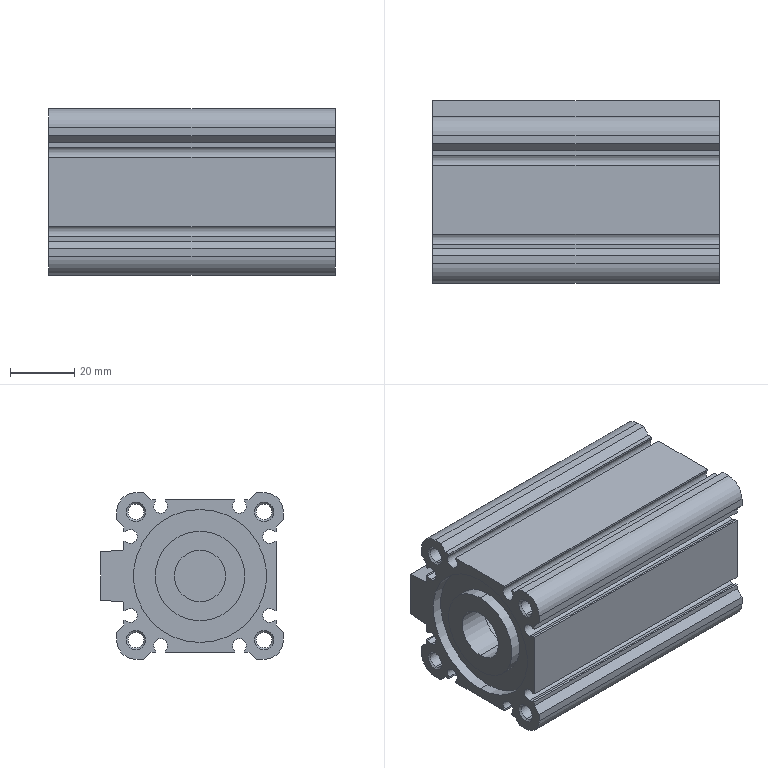Part | STEP file | _CDQ2F40-50-A93(0_0)_BODY.stp | 1 solid | 145 faces | box 89.5 x 57 x 52 mm | volume 126518 mm3 | plane 65 | cylinder 60 | cone 20 | commonest cylinder face diameters 4.26 x18 4.917 x16 6 x8 8.566 x4 12 x4 41.5 x4